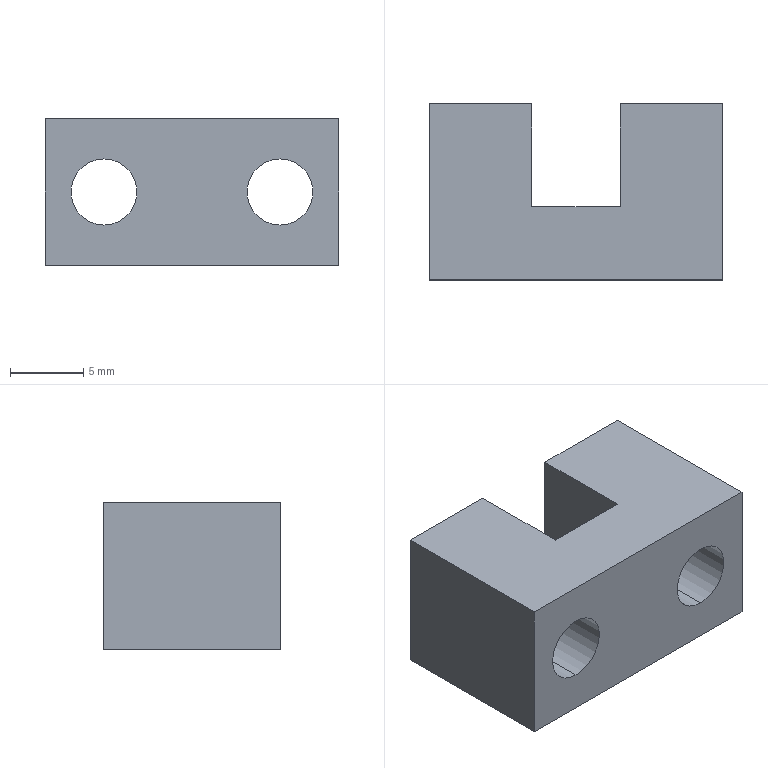Part | STEP file | insert limit | 1 solid | 17 faces | box 20 x 12 x 10 mm | volume 1551 mm3 | plane 11 | cylinder 6 | commonest cylinder face diameters 4.5 x6
STEP:
#1=CARTESIAN_POINT('',(0.,0.,0.));
#2=DIRECTION('',(0.,0.,1.));
#3=DIRECTION('',(1.,0.,0.));
#4=AXIS2_PLACEMENT_3D('',#1,#2,#3);
#5=CARTESIAN_POINT('',(0.,-4.,7.25));
#6=VERTEX_POINT('',#5);
#7=CARTESIAN_POINT('',(0.,-1.,7.25));
#8=VERTEX_POINT('',#7);
#9=CARTESIAN_POINT('',(0.,-12.364,7.25));
#10=DIRECTION('',(0.,1.,0.));
#11=VECTOR('',#10,1.);
#12=LINE('',#9,#11);
#13=CARTESIAN_POINT('',(0.,-12.364,5.));
#14=DIRECTION('',(0.,1.,0.));
#15=DIRECTION('',(0.,0.,1.));
#16=AXIS2_PLACEMENT_3D('',#13,#14,#15);
#17=CYLINDRICAL_SURFACE('',#16,2.25);
#18=CARTESIAN_POINT('',(6.283,0.));
#19=DIRECTION('',(0.,1.));
#20=VECTOR('',#19,1.);
#21=LINE('',#18,#20);
#22=(GEOMETRIC_REPRESENTATION_CONTEXT(2)PARAMETRIC_REPRESENTATION_CONTEXT()REPRESENTATION_CONTEXT('',''));
#23=DEFINITIONAL_REPRESENTATION('',(#21),#22);
#24=PCURVE('',#17,#23);
#25=CARTESIAN_POINT('',(0.,-12.364,5.));
#26=DIRECTION('',(0.,1.,0.));
#27=DIRECTION('',(0.,0.,1.));
#28=AXIS2_PLACEMENT_3D('',#25,#26,#27);
#29=CYLINDRICAL_SURFACE('',#28,2.25);
#30=CARTESIAN_POINT('',(0.,0.));
#31=DIRECTION('',(0.,1.));
#32=VECTOR('',#31,1.);
#33=LINE('',#30,#32);
#34=(GEOMETRIC_REPRESENTATION_CONTEXT(2)PARAMETRIC_REPRESENTATION_CONTEXT()REPRESENTATION_CONTEXT('',''));
#35=DEFINITIONAL_REPRESENTATION('',(#33),#34);
#36=PCURVE('',#29,#35);
#37=SURFACE_CURVE('',#12,(#24,#36),.PCURVE_S1.);
#38=EDGE_CURVE('',#6,#8,#37,.T.);
#39=ORIENTED_EDGE('',*,*,#38,.T.);
#40=CARTESIAN_POINT('',(0.,-1.,2.75));
#41=VERTEX_POINT('',#40);
#42=CARTESIAN_POINT('',(0.,-1.,5.));
#43=DIRECTION('',(0.,1.,0.));
#44=DIRECTION('',(0.,0.,1.));
#45=AXIS2_PLACEMENT_3D('',#42,#43,#44);
#46=CIRCLE('',#45,2.25);
#47=CARTESIAN_POINT('',(0.,11.364));
#48=DIRECTION('',(1.,0.));
#49=VECTOR('',#48,1.);
#50=LINE('',#47,#49);
#51=(GEOMETRIC_REPRESENTATION_CONTEXT(2)PARAMETRIC_REPRESENTATION_CONTEXT()REPRESENTATION_CONTEXT('',''));
#52=DEFINITIONAL_REPRESENTATION('',(#50),#51);
#53=PCURVE('',#17,#52);
#54=CARTESIAN_POINT('',(-3.,-1.,10.));
#55=DIRECTION('',(0.,-1.,0.));
#56=DIRECTION('',(0.,0.,-1.));
#57=AXIS2_PLACEMENT_3D('',#54,#55,#56);
#58=PLANE('',#57);
#59=CARTESIAN_POINT('',(2.75,3.));
#60=CARTESIAN_POINT('',(2.75,6.897));
#61=CARTESIAN_POINT('',(6.125,4.949));
#62=CARTESIAN_POINT('',(9.5,3.));
#63=CARTESIAN_POINT('',(6.125,1.051));
#64=CARTESIAN_POINT('',(2.75,-0.8971));
#65=CARTESIAN_POINT('',(2.75,3.));
#66=(BOUNDED_CURVE()B_SPLINE_CURVE(2,(#59,#60,#61,#62,#63,#64,#65),.UNSPECIFIED.,.T.,.F.)B_SPLINE_CURVE_WITH_KNOTS((1,2,2,2,2,1),(-2.094,0.,2.094,4.189,6.283,8.378),.UNSPECIFIED.)CURVE()GEOMETRIC_REPRESENTATION_ITEM()RATIONAL_B_SPLINE_CURVE((1.,0.5,1.,0.5,1.,0.5,1.))REPRESENTATION_ITEM(''));
#67=(GEOMETRIC_REPRESENTATION_CONTEXT(2)PARAMETRIC_REPRESENTATION_CONTEXT()REPRESENTATION_CONTEXT('',''));
#68=DEFINITIONAL_REPRESENTATION('',(#66),#67);
#69=PCURVE('',#58,#68);
#70=SURFACE_CURVE('',#46,(#53,#69),.PCURVE_S1.);
#71=EDGE_CURVE('',#41,#8,#70,.T.);
#72=ORIENTED_EDGE('',*,*,#71,.F.);
#73=CARTESIAN_POINT('',(0.,-4.,2.75));
#74=VERTEX_POINT('',#73);
#75=CARTESIAN_POINT('',(0.,-12.364,2.75));
#76=DIRECTION('',(0.,1.,0.));
#77=VECTOR('',#76,1.);
#78=LINE('',#75,#77);
#79=CARTESIAN_POINT('',(3.142,0.));
#80=DIRECTION('',(0.,1.));
#81=VECTOR('',#80,1.);
#82=LINE('',#79,#81);
#83=(GEOMETRIC_REPRESENTATION_CONTEXT(2)PARAMETRIC_REPRESENTATION_CONTEXT()REPRESENTATION_CONTEXT('',''));
#84=DEFINITIONAL_REPRESENTATION('',(#82),#83);
#85=PCURVE('',#17,#84);
#86=CARTESIAN_POINT('',(3.142,0.));
#87=DIRECTION('',(0.,1.));
#88=VECTOR('',#87,1.);
#89=LINE('',#86,#88);
#90=(GEOMETRIC_REPRESENTATION_CONTEXT(2)PARAMETRIC_REPRESENTATION_CONTEXT()REPRESENTATION_CONTEXT('',''));
#91=DEFINITIONAL_REPRESENTATION('',(#89),#90);
#92=PCURVE('',#29,#91);
#93=SURFACE_CURVE('',#78,(#85,#92),.PCURVE_S1.);
#94=EDGE_CURVE('',#74,#41,#93,.T.);
#95=ORIENTED_EDGE('',*,*,#94,.F.);
#96=CARTESIAN_POINT('',(0.,-4.,5.));
#97=DIRECTION('',(0.,-1.,0.));
#98=DIRECTION('',(0.,0.,1.));
#99=AXIS2_PLACEMENT_3D('',#96,#97,#98);
#100=CIRCLE('',#99,2.25);
#101=CARTESIAN_POINT('',(6.283,8.364));
#102=DIRECTION('',(-1.,0.));
#103=VECTOR('',#102,1.);
#104=LINE('',#101,#103);
#105=(GEOMETRIC_REPRESENTATION_CONTEXT(2)PARAMETRIC_REPRESENTATION_CONTEXT()REPRESENTATION_CONTEXT('',''));
#106=DEFINITIONAL_REPRESENTATION('',(#104),#105);
#107=PCURVE('',#17,#106);
#108=CARTESIAN_POINT('',(-10.,-4.,10.));
#109=DIRECTION('',(0.,1.,0.));
#110=DIRECTION('',(0.,0.,1.));
#111=AXIS2_PLACEMENT_3D('',#108,#109,#110);
#112=PLANE('',#111);
#113=CARTESIAN_POINT('',(-2.75,10.));
#114=CARTESIAN_POINT('',(-2.75,6.103));
#115=CARTESIAN_POINT('',(-6.125,8.051));
#116=CARTESIAN_POINT('',(-9.5,10.));
#117=CARTESIAN_POINT('',(-6.125,11.949));
#118=CARTESIAN_POINT('',(-2.75,13.897));
#119=CARTESIAN_POINT('',(-2.75,10.));
#120=(BOUNDED_CURVE()B_SPLINE_CURVE(2,(#113,#114,#115,#116,#117,#118,#119),.UNSPECIFIED.,.T.,.F.)B_SPLINE_CURVE_WITH_KNOTS((1,2,2,2,2,1),(-2.094,0.,2.094,4.189,6.283,8.378),.UNSPECIFIED.)CURVE()GEOMETRIC_REPRESENTATION_ITEM()RATIONAL_B_SPLINE_CURVE((1.,0.5,1.,0.5,1.,0.5,1.))REPRESENTATION_ITEM(''));
#121=(GEOMETRIC_REPRESENTATION_CONTEXT(2)PARAMETRIC_REPRESENTATION_CONTEXT()REPRESENTATION_CONTEXT('',''));
#122=DEFINITIONAL_REPRESENTATION('',(#120),#121);
#123=PCURVE('',#112,#122);
#124=SURFACE_CURVE('',#100,(#107,#123),.PCURVE_S1.);
#125=EDGE_CURVE('',#6,#74,#124,.T.);
#126=ORIENTED_EDGE('',*,*,#125,.F.);
#127=EDGE_LOOP('',(#39,#72,#95,#126));
#128=FACE_BOUND('',#127,.F.);
#129=ADVANCED_FACE('',(#128),#17,.F.);
#130=CARTESIAN_POINT('',(6.,6.,2.75));
#131=VERTEX_POINT('',#130);
#132=CARTESIAN_POINT('',(6.,-6.,2.75));
#133=VERTEX_POINT('',#132);
#134=CARTESIAN_POINT('',(6.,6.,2.75));
#135=DIRECTION('',(0.,-1.,0.));
#136=VECTOR('',#135,1.);
#137=LINE('',#134,#136);
#138=CARTESIAN_POINT('',(6.,6.,5.));
#139=DIRECTION('',(0.,-1.,0.));
#140=DIRECTION('',(0.,0.,-1.));
#141=AXIS2_PLACEMENT_3D('',#138,#139,#140);
#142=CYLINDRICAL_SURFACE('',#141,2.25);
#143=CARTESIAN_POINT('',(6.283,0.));
#144=DIRECTION('',(0.,1.));
#145=VECTOR('',#144,1.);
#146=LINE('',#143,#145);
#147=(GEOMETRIC_REPRESENTATION_CONTEXT(2)PARAMETRIC_REPRESENTATION_CONTEXT()REPRESENTATION_CONTEXT('',''));
#148=DEFINITIONAL_REPRESENTATION('',(#146),#147);
#149=PCURVE('',#142,#148);
#150=CARTESIAN_POINT('',(6.,6.,5.));
#151=DIRECTION('',(0.,-1.,0.));
#152=DIRECTION('',(0.,0.,-1.));
#153=AXIS2_PLACEMENT_3D('',#150,#151,#152);
#154=CYLINDRICAL_SURFACE('',#153,2.25);
#155=CARTESIAN_POINT('',(0.,0.));
#156=DIRECTION('',(0.,1.));
#157=VECTOR('',#156,1.);
#158=LINE('',#155,#157);
#159=(GEOMETRIC_REPRESENTATION_CONTEXT(2)PARAMETRIC_REPRESENTATION_CONTEXT()REPRESENTATION_CONTEXT('',''));
#160=DEFINITIONAL_REPRESENTATION('',(#158),#159);
#161=PCURVE('',#154,#160);
#162=SURFACE_CURVE('',#137,(#149,#161),.PCURVE_S1.);
#163=EDGE_CURVE('',#131,#133,#162,.T.);
#164=ORIENTED_EDGE('',*,*,#163,.T.);
#165=CARTESIAN_POINT('',(6.,-6.,7.25));
#166=VERTEX_POINT('',#165);
#167=CARTESIAN_POINT('',(6.,-6.,5.));
#168=DIRECTION('',(0.,-1.,0.));
#169=DIRECTION('',(0.,0.,-1.));
#170=AXIS2_PLACEMENT_3D('',#167,#168,#169);
#171=CIRCLE('',#170,2.25);
#172=CARTESIAN_POINT('',(0.,12.));
#173=DIRECTION('',(1.,0.));
#174=VECTOR('',#173,1.);
#175=LINE('',#172,#174);
#176=(GEOMETRIC_REPRESENTATION_CONTEXT(2)PARAMETRIC_REPRESENTATION_CONTEXT()REPRESENTATION_CONTEXT('',''));
#177=DEFINITIONAL_REPRESENTATION('',(#175),#176);
#178=PCURVE('',#142,#177);
#179=CARTESIAN_POINT('',(-10.,-6.,10.));
#180=DIRECTION('',(0.,1.,0.));
#181=DIRECTION('',(0.,0.,1.));
#182=AXIS2_PLACEMENT_3D('',#179,#180,#181);
#183=PLANE('',#182);
#184=CARTESIAN_POINT('',(-7.25,16.));
#185=CARTESIAN_POINT('',(-7.25,19.897));
#186=CARTESIAN_POINT('',(-3.875,17.949));
#187=CARTESIAN_POINT('',(-0.5,16.));
#188=CARTESIAN_POINT('',(-3.875,14.051));
#189=CARTESIAN_POINT('',(-7.25,12.103));
#190=CARTESIAN_POINT('',(-7.25,16.));
#191=(BOUNDED_CURVE()B_SPLINE_CURVE(2,(#184,#185,#186,#187,#188,#189,#190),.UNSPECIFIED.,.T.,.F.)B_SPLINE_CURVE_WITH_KNOTS((1,2,2,2,2,1),(-2.094,0.,2.094,4.189,6.283,8.378),.UNSPECIFIED.)CURVE()GEOMETRIC_REPRESENTATION_ITEM()RATIONAL_B_SPLINE_CURVE((1.,0.5,1.,0.5,1.,0.5,1.))REPRESENTATION_ITEM(''));
#192=(GEOMETRIC_REPRESENTATION_CONTEXT(2)PARAMETRIC_REPRESENTATION_CONTEXT()REPRESENTATION_CONTEXT('',''));
#193=DEFINITIONAL_REPRESENTATION('',(#191),#192);
#194=PCURVE('',#183,#193);
#195=SURFACE_CURVE('',#171,(#178,#194),.PCURVE_S1.);
#196=EDGE_CURVE('',#166,#133,#195,.T.);
#197=ORIENTED_EDGE('',*,*,#196,.F.);
#198=CARTESIAN_POINT('',(6.,6.,7.25));
#199=VERTEX_POINT('',#198);
#200=CARTESIAN_POINT('',(6.,6.,7.25));
#201=DIRECTION('',(0.,-1.,0.));
#202=VECTOR('',#201,1.);
#203=LINE('',#200,#202);
#204=CARTESIAN_POINT('',(3.142,0.));
#205=DIRECTION('',(0.,1.));
#206=VECTOR('',#205,1.);
#207=LINE('',#204,#206);
#208=(GEOMETRIC_REPRESENTATION_CONTEXT(2)PARAMETRIC_REPRESENTATION_CONTEXT()REPRESENTATION_CONTEXT('',''));
#209=DEFINITIONAL_REPRESENTATION('',(#207),#208);
#210=PCURVE('',#142,#209);
#211=CARTESIAN_POINT('',(3.142,0.));
#212=DIRECTION('',(0.,1.));
#213=VECTOR('',#212,1.);
#214=LINE('',#211,#213);
#215=(GEOMETRIC_REPRESENTATION_CONTEXT(2)PARAMETRIC_REPRESENTATION_CONTEXT()REPRESENTATION_CONTEXT('',''));
#216=DEFINITIONAL_REPRESENTATION('',(#214),#215);
#217=PCURVE('',#154,#216);
#218=SURFACE_CURVE('',#203,(#210,#217),.PCURVE_S1.);
#219=EDGE_CURVE('',#199,#166,#218,.T.);
#220=ORIENTED_EDGE('',*,*,#219,.F.);
#221=CARTESIAN_POINT('',(6.,6.,5.));
#222=DIRECTION('',(0.,-1.,0.));
#223=DIRECTION('',(0.,0.,-1.));
#224=AXIS2_PLACEMENT_3D('',#221,#222,#223);
#225=CIRCLE('',#224,2.25);
#226=CARTESIAN_POINT('',(0.,0.));
#227=DIRECTION('',(1.,0.));
#228=VECTOR('',#227,1.);
#229=LINE('',#226,#228);
#230=(GEOMETRIC_REPRESENTATION_CONTEXT(2)PARAMETRIC_REPRESENTATION_CONTEXT()REPRESENTATION_CONTEXT('',''));
#231=DEFINITIONAL_REPRESENTATION('',(#229),#230);
#232=PCURVE('',#142,#231);
#233=CARTESIAN_POINT('',(3.,6.,10.));
#234=DIRECTION('',(0.,-1.,0.));
#235=DIRECTION('',(0.,0.,-1.));
#236=AXIS2_PLACEMENT_3D('',#233,#234,#235);
#237=PLANE('',#236);
#238=CARTESIAN_POINT('',(5.,3.));
#239=DIRECTION('',(1.,0.));
#240=AXIS2_PLACEMENT_2D('',#238,#239);
#241=CIRCLE('',#240,2.25);
#242=(GEOMETRIC_REPRESENTATION_CONTEXT(2)PARAMETRIC_REPRESENTATION_CONTEXT()REPRESENTATION_CONTEXT('',''));
#243=DEFINITIONAL_REPRESENTATION('',(#241),#242);
#244=PCURVE('',#237,#243);
#245=SURFACE_CURVE('',#225,(#232,#244),.PCURVE_S1.);
#246=EDGE_CURVE('',#199,#131,#245,.T.);
#247=ORIENTED_EDGE('',*,*,#246,.T.);
#248=EDGE_LOOP('',(#164,#197,#220,#247));
#249=FACE_BOUND('',#248,.F.);
#250=ADVANCED_FACE('',(#249),#142,.F.);
#251=CARTESIAN_POINT('',(-6.,6.,2.75));
#252=VERTEX_POINT('',#251);
#253=CARTESIAN_POINT('',(-6.,-6.,2.75));
#254=VERTEX_POINT('',#253);
#255=CARTESIAN_POINT('',(-6.,6.,2.75));
#256=DIRECTION('',(0.,-1.,0.));
#257=VECTOR('',#256,1.);
#258=LINE('',#255,#257);
#259=CARTESIAN_POINT('',(-6.,6.,5.));
#260=DIRECTION('',(0.,-1.,0.));
#261=DIRECTION('',(0.,0.,-1.));
#262=AXIS2_PLACEMENT_3D('',#259,#260,#261);
#263=CYLINDRICAL_SURFACE('',#262,2.25);
#264=CARTESIAN_POINT('',(6.283,0.));
#265=DIRECTION('',(0.,1.));
#266=VECTOR('',#265,1.);
#267=LINE('',#264,#266);
#268=(GEOMETRIC_REPRESENTATION_CONTEXT(2)PARAMETRIC_REPRESENTATION_CONTEXT()REPRESENTATION_CONTEXT('',''));
#269=DEFINITIONAL_REPRESENTATION('',(#267),#268);
#270=PCURVE('',#263,#269);
#271=CARTESIAN_POINT('',(-6.,6.,5.));
#272=DIRECTION('',(0.,-1.,0.));
#273=DIRECTION('',(0.,0.,-1.));
#274=AXIS2_PLACEMENT_3D('',#271,#272,#273);
#275=CYLINDRICAL_SURFACE('',#274,2.25);
#276=CARTESIAN_POINT('',(0.,0.));
#277=DIRECTION('',(0.,1.));
#278=VECTOR('',#277,1.);
#279=LINE('',#276,#278);
#280=(GEOMETRIC_REPRESENTATION_CONTEXT(2)PARAMETRIC_REPRESENTATION_CONTEXT()REPRESENTATION_CONTEXT('',''));
#281=DEFINITIONAL_REPRESENTATION('',(#279),#280);
#282=PCURVE('',#275,#281);
#283=SURFACE_CURVE('',#258,(#270,#282),.PCURVE_S1.);
#284=EDGE_CURVE('',#252,#254,#283,.T.);
#285=ORIENTED_EDGE('',*,*,#284,.T.);
#286=CARTESIAN_POINT('',(-6.,-6.,7.25));
#287=VERTEX_POINT('',#286);
#288=CARTESIAN_POINT('',(-6.,-6.,5.));
#289=DIRECTION('',(0.,-1.,0.));
#290=DIRECTION('',(0.,0.,-1.));
#291=AXIS2_PLACEMENT_3D('',#288,#289,#290);
#292=CIRCLE('',#291,2.25);
#293=CARTESIAN_POINT('',(0.,12.));
#294=DIRECTION('',(1.,0.));
#295=VECTOR('',#294,1.);
#296=LINE('',#293,#295);
#297=(GEOMETRIC_REPRESENTATION_CONTEXT(2)PARAMETRIC_REPRESENTATION_CONTEXT()REPRESENTATION_CONTEXT('',''));
#298=DEFINITIONAL_REPRESENTATION('',(#296),#297);
#299=PCURVE('',#263,#298);
#300=CARTESIAN_POINT('',(-7.25,4.));
#301=CARTESIAN_POINT('',(-7.25,7.897));
#302=CARTESIAN_POINT('',(-3.875,5.949));
#303=CARTESIAN_POINT('',(-0.5,4.));
#304=CARTESIAN_POINT('',(-3.875,2.051));
#305=CARTESIAN_POINT('',(-7.25,0.1029));
#306=CARTESIAN_POINT('',(-7.25,4.));
#307=(BOUNDED_CURVE()B_SPLINE_CURVE(2,(#300,#301,#302,#303,#304,#305,#306),.UNSPECIFIED.,.T.,.F.)B_SPLINE_CURVE_WITH_KNOTS((1,2,2,2,2,1),(-2.094,0.,2.094,4.189,6.283,8.378),.UNSPECIFIED.)CURVE()GEOMETRIC_REPRESENTATION_ITEM()RATIONAL_B_SPLINE_CURVE((1.,0.5,1.,0.5,1.,0.5,1.))REPRESENTATION_ITEM(''));
#308=(GEOMETRIC_REPRESENTATION_CONTEXT(2)PARAMETRIC_REPRESENTATION_CONTEXT()REPRESENTATION_CONTEXT('',''));
#309=DEFINITIONAL_REPRESENTATION('',(#307),#308);
#310=PCURVE('',#183,#309);
#311=SURFACE_CURVE('',#292,(#299,#310),.PCURVE_S1.);
#312=EDGE_CURVE('',#287,#254,#311,.T.);
#313=ORIENTED_EDGE('',*,*,#312,.F.);
#314=CARTESIAN_POINT('',(-6.,6.,7.25));
#315=VERTEX_POINT('',#314);
#316=CARTESIAN_POINT('',(-6.,6.,7.25));
#317=DIRECTION('',(0.,-1.,0.));
#318=VECTOR('',#317,1.);
#319=LINE('',#316,#318);
#320=CARTESIAN_POINT('',(3.142,0.));
#321=DIRECTION('',(0.,1.));
#322=VECTOR('',#321,1.);
#323=LINE('',#320,#322);
#324=(GEOMETRIC_REPRESENTATION_CONTEXT(2)PARAMETRIC_REPRESENTATION_CONTEXT()REPRESENTATION_CONTEXT('',''));
#325=DEFINITIONAL_REPRESENTATION('',(#323),#324);
#326=PCURVE('',#263,#325);
#327=CARTESIAN_POINT('',(3.142,0.));
#328=DIRECTION('',(0.,1.));
#329=VECTOR('',#328,1.);
#330=LINE('',#327,#329);
#331=(GEOMETRIC_REPRESENTATION_CONTEXT(2)PARAMETRIC_REPRESENTATION_CONTEXT()REPRESENTATION_CONTEXT('',''));
#332=DEFINITIONAL_REPRESENTATION('',(#330),#331);
#333=PCURVE('',#275,#332);
#334=SURFACE_CURVE('',#319,(#326,#333),.PCURVE_S1.);
#335=EDGE_CURVE('',#315,#287,#334,.T.);
#336=ORIENTED_EDGE('',*,*,#335,.F.);
#337=CARTESIAN_POINT('',(-6.,6.,5.));
#338=DIRECTION('',(0.,-1.,0.));
#339=DIRECTION('',(0.,0.,-1.));
#340=AXIS2_PLACEMENT_3D('',#337,#338,#339);
#341=CIRCLE('',#340,2.25);
#342=CARTESIAN_POINT('',(0.,0.));
#343=DIRECTION('',(1.,0.));
#344=VECTOR('',#343,1.);
#345=LINE('',#342,#344);
#346=(GEOMETRIC_REPRESENTATION_CONTEXT(2)PARAMETRIC_REPRESENTATION_CONTEXT()REPRESENTATION_CONTEXT('',''));
#347=DEFINITIONAL_REPRESENTATION('',(#345),#346);
#348=PCURVE('',#263,#347);
#349=CARTESIAN_POINT('',(-10.,6.,10.));
#350=DIRECTION('',(0.,-1.,0.));
#351=DIRECTION('',(0.,0.,-1.));
#352=AXIS2_PLACEMENT_3D('',#349,#350,#351);
#353=PLANE('',#352);
#354=CARTESIAN_POINT('',(5.,4.));
#355=DIRECTION('',(1.,0.));
#356=AXIS2_PLACEMENT_2D('',#354,#355);
#357=CIRCLE('',#356,2.25);
#358=(GEOMETRIC_REPRESENTATION_CONTEXT(2)PARAMETRIC_REPRESENTATION_CONTEXT()REPRESENTATION_CONTEXT('',''));
#359=DEFINITIONAL_REPRESENTATION('',(#357),#358);
#360=PCURVE('',#353,#359);
#361=SURFACE_CURVE('',#341,(#348,#360),.PCURVE_S1.);
#362=EDGE_CURVE('',#315,#252,#361,.T.);
#363=ORIENTED_EDGE('',*,*,#362,.T.);
#364=EDGE_LOOP('',(#285,#313,#336,#363));
#365=FACE_BOUND('',#364,.F.);
#366=ADVANCED_FACE('',(#365),#263,.F.);
#367=CARTESIAN_POINT('',(6.,6.,5.));
#368=DIRECTION('',(0.,-1.,0.));
#369=DIRECTION('',(0.,0.,-1.));
#370=AXIS2_PLACEMENT_3D('',#367,#368,#369);
#371=CIRCLE('',#370,2.25);
#372=CARTESIAN_POINT('',(5.,3.));
#373=DIRECTION('',(1.,0.));
#374=AXIS2_PLACEMENT_2D('',#372,#373);
#375=CIRCLE('',#374,2.25);
#376=(GEOMETRIC_REPRESENTATION_CONTEXT(2)PARAMETRIC_REPRESENTATION_CONTEXT()REPRESENTATION_CONTEXT('',''));
#377=DEFINITIONAL_REPRESENTATION('',(#375),#376);
#378=PCURVE('',#237,#377);
#379=CARTESIAN_POINT('',(0.,0.));
#380=DIRECTION('',(1.,0.));
#381=VECTOR('',#380,1.);
#382=LINE('',#379,#381);
#383=(GEOMETRIC_REPRESENTATION_CONTEXT(2)PARAMETRIC_REPRESENTATION_CONTEXT()REPRESENTATION_CONTEXT('',''));
#384=DEFINITIONAL_REPRESENTATION('',(#382),#383);
#385=PCURVE('',#154,#384);
#386=SURFACE_CURVE('',#371,(#378,#385),.PCURVE_S1.);
#387=EDGE_CURVE('',#131,#199,#386,.T.);
#388=ORIENTED_EDGE('',*,*,#387,.T.);
#389=ORIENTED_EDGE('',*,*,#246,.T.);
#390=EDGE_LOOP('',(#388,#389));
#391=FACE_BOUND('',#390,.T.);
#392=CARTESIAN_POINT('',(10.,6.,0.));
#393=VERTEX_POINT('',#392);
#394=CARTESIAN_POINT('',(3.,6.,0.));
#395=VERTEX_POINT('',#394);
#396=CARTESIAN_POINT('',(3.,6.,0.));
#397=DIRECTION('',(-1.,0.,0.));
#398=VECTOR('',#397,1.);
#399=LINE('',#396,#398);
#400=CARTESIAN_POINT('',(10.,0.));
#401=DIRECTION('',(0.,-1.));
#402=VECTOR('',#401,1.);
#403=LINE('',#400,#402);
#404=(GEOMETRIC_REPRESENTATION_CONTEXT(2)PARAMETRIC_REPRESENTATION_CONTEXT()REPRESENTATION_CONTEXT('',''));
#405=DEFINITIONAL_REPRESENTATION('',(#403),#404);
#406=PCURVE('',#237,#405);
#407=CARTESIAN_POINT('',(10.,6.,0.));
#408=DIRECTION('',(0.,0.,1.));
#409=DIRECTION('',(1.,0.,0.));
#410=AXIS2_PLACEMENT_3D('',#407,#408,#409);
#411=PLANE('',#410);
#412=CARTESIAN_POINT('',(-7.,0.));
#413=DIRECTION('',(-1.,0.));
#414=VECTOR('',#413,1.);
#415=LINE('',#412,#414);
#416=(GEOMETRIC_REPRESENTATION_CONTEXT(2)PARAMETRIC_REPRESENTATION_CONTEXT()REPRESENTATION_CONTEXT('',''));
#417=DEFINITIONAL_REPRESENTATION('',(#415),#416);
#418=PCURVE('',#411,#417);
#419=SURFACE_CURVE('',#399,(#406,#418),.PCURVE_S1.);
#420=EDGE_CURVE('',#393,#395,#419,.T.);
#421=ORIENTED_EDGE('',*,*,#420,.T.);
#422=CARTESIAN_POINT('',(3.,6.,10.));
#423=VERTEX_POINT('',#422);
#424=CARTESIAN_POINT('',(3.,6.,10.));
#425=DIRECTION('',(0.,0.,-1.));
#426=VECTOR('',#425,1.);
#427=LINE('',#424,#426);
#428=CARTESIAN_POINT('',(0.,0.));
#429=DIRECTION('',(1.,0.));
#430=VECTOR('',#429,1.);
#431=LINE('',#428,#430);
#432=(GEOMETRIC_REPRESENTATION_CONTEXT(2)PARAMETRIC_REPRESENTATION_CONTEXT()REPRESENTATION_CONTEXT('',''));
#433=DEFINITIONAL_REPRESENTATION('',(#431),#432);
#434=PCURVE('',#237,#433);
#435=CARTESIAN_POINT('',(3.,6.,10.));
#436=DIRECTION('',(1.,0.,0.));
#437=DIRECTION('',(0.,1.,0.));
#438=AXIS2_PLACEMENT_3D('',#435,#436,#437);
#439=PLANE('',#438);
#440=CARTESIAN_POINT('',(0.,0.));
#441=DIRECTION('',(0.,-1.));
#442=VECTOR('',#441,1.);
#443=LINE('',#440,#442);
#444=(GEOMETRIC_REPRESENTATION_CONTEXT(2)PARAMETRIC_REPRESENTATION_CONTEXT()REPRESENTATION_CONTEXT('',''));
#445=DEFINITIONAL_REPRESENTATION('',(#443),#444);
#446=PCURVE('',#439,#445);
#447=SURFACE_CURVE('',#427,(#434,#446),.PCURVE_S1.);
#448=EDGE_CURVE('',#423,#395,#447,.T.);
#449=ORIENTED_EDGE('',*,*,#448,.F.);
#450=CARTESIAN_POINT('',(10.,6.,10.));
#451=VERTEX_POINT('',#450);
#452=CARTESIAN_POINT('',(3.,6.,10.));
#453=DIRECTION('',(-1.,0.,0.));
#454=VECTOR('',#453,1.);
#455=LINE('',#452,#454);
#456=CARTESIAN_POINT('',(0.,0.));
#457=DIRECTION('',(0.,-1.));
#458=VECTOR('',#457,1.);
#459=LINE('',#456,#458);
#460=(GEOMETRIC_REPRESENTATION_CONTEXT(2)PARAMETRIC_REPRESENTATION_CONTEXT()REPRESENTATION_CONTEXT('',''));
#461=DEFINITIONAL_REPRESENTATION('',(#459),#460);
#462=PCURVE('',#237,#461);
#463=CARTESIAN_POINT('',(10.,6.,10.));
#464=DIRECTION('',(0.,0.,1.));
#465=DIRECTION('',(1.,0.,0.));
#466=AXIS2_PLACEMENT_3D('',#463,#464,#465);
#467=PLANE('',#466);
#468=CARTESIAN_POINT('',(-7.,0.));
#469=DIRECTION('',(-1.,0.));
#470=VECTOR('',#469,1.);
#471=LINE('',#468,#470);
#472=(GEOMETRIC_REPRESENTATION_CONTEXT(2)PARAMETRIC_REPRESENTATION_CONTEXT()REPRESENTATION_CONTEXT('',''));
#473=DEFINITIONAL_REPRESENTATION('',(#471),#472);
#474=PCURVE('',#467,#473);
#475=SURFACE_CURVE('',#455,(#462,#474),.PCURVE_S1.);
#476=EDGE_CURVE('',#451,#423,#475,.T.);
#477=ORIENTED_EDGE('',*,*,#476,.F.);
#478=CARTESIAN_POINT('',(10.,6.,10.));
#479=DIRECTION('',(0.,0.,-1.));
#480=VECTOR('',#479,1.);
#481=LINE('',#478,#480);
#482=CARTESIAN_POINT('',(0.,7.));
#483=DIRECTION('',(1.,0.));
#484=VECTOR('',#483,1.);
#485=LINE('',#482,#484);
#486=(GEOMETRIC_REPRESENTATION_CONTEXT(2)PARAMETRIC_REPRESENTATION_CONTEXT()REPRESENTATION_CONTEXT('',''));
#487=DEFINITIONAL_REPRESENTATION('',(#485),#486);
#488=PCURVE('',#237,#487);
#489=CARTESIAN_POINT('',(10.,-6.,10.));
#490=DIRECTION('',(-1.,0.,0.));
#491=DIRECTION('',(0.,0.,1.));
#492=AXIS2_PLACEMENT_3D('',#489,#490,#491);
#493=PLANE('',#492);
#494=CARTESIAN_POINT('',(0.,12.));
#495=DIRECTION('',(-1.,0.));
#496=VECTOR('',#495,1.);
#497=LINE('',#494,#496);
#498=(GEOMETRIC_REPRESENTATION_CONTEXT(2)PARAMETRIC_REPRESENTATION_CONTEXT()REPRESENTATION_CONTEXT('',''));
#499=DEFINITIONAL_REPRESENTATION('',(#497),#498);
#500=PCURVE('',#493,#499);
#501=SURFACE_CURVE('',#481,(#488,#500),.PCURVE_S1.);
#502=EDGE_CURVE('',#451,#393,#501,.T.);
#503=ORIENTED_EDGE('',*,*,#502,.T.);
#504=EDGE_LOOP('',(#421,#449,#477,#503));
#505=FACE_BOUND('',#504,.T.);
#506=ADVANCED_FACE('',(#391,#505),#237,.F.);
#507=CARTESIAN_POINT('',(3.,-1.,0.));
#508=VERTEX_POINT('',#507);
#509=CARTESIAN_POINT('',(3.,6.,0.));
#510=DIRECTION('',(0.,-1.,0.));
#511=VECTOR('',#510,1.);
#512=LINE('',#509,#511);
#513=CARTESIAN_POINT('',(0.,-10.));
#514=DIRECTION('',(-1.,0.));
#515=VECTOR('',#514,1.);
#516=LINE('',#513,#515);
#517=(GEOMETRIC_REPRESENTATION_CONTEXT(2)PARAMETRIC_REPRESENTATION_CONTEXT()REPRESENTATION_CONTEXT('',''));
#518=DEFINITIONAL_REPRESENTATION('',(#516),#517);
#519=PCURVE('',#439,#518);
#520=CARTESIAN_POINT('',(-7.,0.));
#521=DIRECTION('',(0.,-1.));
#522=VECTOR('',#521,1.);
#523=LINE('',#520,#522);
#524=(GEOMETRIC_REPRESENTATION_CONTEXT(2)PARAMETRIC_REPRESENTATION_CONTEXT()REPRESENTATION_CONTEXT('',''));
#525=DEFINITIONAL_REPRESENTATION('',(#523),#524);
#526=PCURVE('',#411,#525);
#527=SURFACE_CURVE('',#512,(#519,#526),.PCURVE_S1.);
#528=EDGE_CURVE('',#395,#508,#527,.T.);
#529=ORIENTED_EDGE('',*,*,#528,.T.);
#530=CARTESIAN_POINT('',(3.,-1.,10.));
#531=VERTEX_POINT('',#530);
#532=CARTESIAN_POINT('',(3.,-1.,10.));
#533=DIRECTION('',(0.,0.,-1.));
#534=VECTOR('',#533,1.);
#535=LINE('',#532,#534);
#536=CARTESIAN_POINT('',(-7.,0.));
#537=DIRECTION('',(0.,-1.));
#538=VECTOR('',#537,1.);
#539=LINE('',#536,#538);
#540=(GEOMETRIC_REPRESENTATION_CONTEXT(2)PARAMETRIC_REPRESENTATION_CONTEXT()REPRESENTATION_CONTEXT('',''));
#541=DEFINITIONAL_REPRESENTATION('',(#539),#540);
#542=PCURVE('',#439,#541);
#543=CARTESIAN_POINT('',(0.,6.));
#544=DIRECTION('',(1.,0.));
#545=VECTOR('',#544,1.);
#546=LINE('',#543,#545);
#547=(GEOMETRIC_REPRESENTATION_CONTEXT(2)PARAMETRIC_REPRESENTATION_CONTEXT()REPRESENTATION_CONTEXT('',''));
#548=DEFINITIONAL_REPRESENTATION('',(#546),#547);
#549=PCURVE('',#58,#548);
#550=SURFACE_CURVE('',#535,(#542,#549),.PCURVE_S1.);
#551=EDGE_CURVE('',#531,#508,#550,.T.);
#552=ORIENTED_EDGE('',*,*,#551,.F.);
#553=CARTESIAN_POINT('',(3.,6.,10.));
#554=DIRECTION('',(0.,-1.,0.));
#555=VECTOR('',#554,1.);
#556=LINE('',#553,#555);
#557=CARTESIAN_POINT('',(0.,0.));
#558=DIRECTION('',(-1.,0.));
#559=VECTOR('',#558,1.);
#560=LINE('',#557,#559);
#561=(GEOMETRIC_REPRESENTATION_CONTEXT(2)PARAMETRIC_REPRESENTATION_CONTEXT()REPRESENTATION_CONTEXT('',''));
#562=DEFINITIONAL_REPRESENTATION('',(#560),#561);
#563=PCURVE('',#439,#562);
#564=CARTESIAN_POINT('',(-7.,0.));
#565=DIRECTION('',(0.,-1.));
#566=VECTOR('',#565,1.);
#567=LINE('',#564,#566);
#568=(GEOMETRIC_REPRESENTATION_CONTEXT(2)PARAMETRIC_REPRESENTATION_CONTEXT()REPRESENTATION_CONTEXT('',''));
#569=DEFINITIONAL_REPRESENTATION('',(#567),#568);
#570=PCURVE('',#467,#569);
#571=SURFACE_CURVE('',#556,(#563,#570),.PCURVE_S1.);
#572=EDGE_CURVE('',#423,#531,#571,.T.);
#573=ORIENTED_EDGE('',*,*,#572,.F.);
#574=ORIENTED_EDGE('',*,*,#448,.T.);
#575=EDGE_LOOP('',(#529,#552,#573,#574));
#576=FACE_BOUND('',#575,.T.);
#577=ADVANCED_FACE('',(#576),#439,.F.);
#578=CARTESIAN_POINT('',(0.,-1.,5.));
#579=DIRECTION('',(0.,1.,0.));
#580=DIRECTION('',(0.,0.,1.));
#581=AXIS2_PLACEMENT_3D('',#578,#579,#580);
#582=CIRCLE('',#581,2.25);
#583=CARTESIAN_POINT('',(2.75,3.));
#584=CARTESIAN_POINT('',(2.75,6.897));
#585=CARTESIAN_POINT('',(6.125,4.949));
#586=CARTESIAN_POINT('',(9.5,3.));
#587=CARTESIAN_POINT('',(6.125,1.051));
#588=CARTESIAN_POINT('',(2.75,-0.8971));
#589=CARTESIAN_POINT('',(2.75,3.));
#590=(BOUNDED_CURVE()B_SPLINE_CURVE(2,(#583,#584,#585,#586,#587,#588,#589),.UNSPECIFIED.,.T.,.F.)B_SPLINE_CURVE_WITH_KNOTS((1,2,2,2,2,1),(-2.094,0.,2.094,4.189,6.283,8.378),.UNSPECIFIED.)CURVE()GEOMETRIC_REPRESENTATION_ITEM()RATIONAL_B_SPLINE_CURVE((1.,0.5,1.,0.5,1.,0.5,1.))REPRESENTATION_ITEM(''));
#591=(GEOMETRIC_REPRESENTATION_CONTEXT(2)PARAMETRIC_REPRESENTATION_CONTEXT()REPRESENTATION_CONTEXT('',''));
#592=DEFINITIONAL_REPRESENTATION('',(#590),#591);
#593=PCURVE('',#58,#592);
#594=CARTESIAN_POINT('',(0.,11.364));
#595=DIRECTION('',(1.,0.));
#596=VECTOR('',#595,1.);
#597=LINE('',#594,#596);
#598=(GEOMETRIC_REPRESENTATION_CONTEXT(2)PARAMETRIC_REPRESENTATION_CONTEXT()REPRESENTATION_CONTEXT('',''));
#599=DEFINITIONAL_REPRESENTATION('',(#597),#598);
#600=PCURVE('',#29,#599);
#601=SURFACE_CURVE('',#582,(#593,#600),.PCURVE_S1.);
#602=EDGE_CURVE('',#8,#41,#601,.T.);
#603=ORIENTED_EDGE('',*,*,#602,.F.);
#604=ORIENTED_EDGE('',*,*,#71,.F.);
#605=EDGE_LOOP('',(#603,#604));
#606=FACE_BOUND('',#605,.T.);
#607=CARTESIAN_POINT('',(-3.,-1.,0.));
#608=VERTEX_POINT('',#607);
#609=CARTESIAN_POINT('',(-3.,-1.,0.));
#610=DIRECTION('',(-1.,0.,0.));
#611=VECTOR('',#610,1.);
#612=LINE('',#609,#611);
#613=CARTESIAN_POINT('',(10.,0.));
#614=DIRECTION('',(0.,-1.));
#615=VECTOR('',#614,1.);
#616=LINE('',#613,#615);
#617=(GEOMETRIC_REPRESENTATION_CONTEXT(2)PARAMETRIC_REPRESENTATION_CONTEXT()REPRESENTATION_CONTEXT('',''));
#618=DEFINITIONAL_REPRESENTATION('',(#616),#617);
#619=PCURVE('',#58,#618);
#620=CARTESIAN_POINT('',(-13.,-7.));
#621=DIRECTION('',(-1.,0.));
#622=VECTOR('',#621,1.);
#623=LINE('',#620,#622);
#624=(GEOMETRIC_REPRESENTATION_CONTEXT(2)PARAMETRIC_REPRESENTATION_CONTEXT()REPRESENTATION_CONTEXT('',''));
#625=DEFINITIONAL_REPRESENTATION('',(#623),#624);
#626=PCURVE('',#411,#625);
#627=SURFACE_CURVE('',#612,(#619,#626),.PCURVE_S1.);
#628=EDGE_CURVE('',#508,#608,#627,.T.);
#629=ORIENTED_EDGE('',*,*,#628,.T.);
#630=CARTESIAN_POINT('',(-3.,-1.,10.));
#631=VERTEX_POINT('',#630);
#632=CARTESIAN_POINT('',(-3.,-1.,10.));
#633=DIRECTION('',(0.,0.,-1.));
#634=VECTOR('',#633,1.);
#635=LINE('',#632,#634);
#636=CARTESIAN_POINT('',(0.,0.));
#637=DIRECTION('',(1.,0.));
#638=VECTOR('',#637,1.);
#639=LINE('',#636,#638);
#640=(GEOMETRIC_REPRESENTATION_CONTEXT(2)PARAMETRIC_REPRESENTATION_CONTEXT()REPRESENTATION_CONTEXT('',''));
#641=DEFINITIONAL_REPRESENTATION('',(#639),#640);
#642=PCURVE('',#58,#641);
#643=CARTESIAN_POINT('',(-3.,6.,10.));
#644=DIRECTION('',(-1.,0.,0.));
#645=DIRECTION('',(0.,-1.,0.));
#646=AXIS2_PLACEMENT_3D('',#643,#644,#645);
#647=PLANE('',#646);
#648=CARTESIAN_POINT('',(7.,0.));
#649=DIRECTION('',(0.,-1.));
#650=VECTOR('',#649,1.);
#651=LINE('',#648,#650);
#652=(GEOMETRIC_REPRESENTATION_CONTEXT(2)PARAMETRIC_REPRESENTATION_CONTEXT()REPRESENTATION_CONTEXT('',''));
#653=DEFINITIONAL_REPRESENTATION('',(#651),#652);
#654=PCURVE('',#647,#653);
#655=SURFACE_CURVE('',#635,(#642,#654),.PCURVE_S1.);
#656=EDGE_CURVE('',#631,#608,#655,.T.);
#657=ORIENTED_EDGE('',*,*,#656,.F.);
#658=CARTESIAN_POINT('',(-3.,-1.,10.));
#659=DIRECTION('',(-1.,0.,0.));
#660=VECTOR('',#659,1.);
#661=LINE('',#658,#660);
#662=CARTESIAN_POINT('',(0.,0.));
#663=DIRECTION('',(0.,-1.));
#664=VECTOR('',#663,1.);
#665=LINE('',#662,#664);
#666=(GEOMETRIC_REPRESENTATION_CONTEXT(2)PARAMETRIC_REPRESENTATION_CONTEXT()REPRESENTATION_CONTEXT('',''));
#667=DEFINITIONAL_REPRESENTATION('',(#665),#666);
#668=PCURVE('',#58,#667);
#669=CARTESIAN_POINT('',(-13.,-7.));
#670=DIRECTION('',(-1.,0.));
#671=VECTOR('',#670,1.);
#672=LINE('',#669,#671);
#673=(GEOMETRIC_REPRESENTATION_CONTEXT(2)PARAMETRIC_REPRESENTATION_CONTEXT()REPRESENTATION_CONTEXT('',''));
#674=DEFINITIONAL_REPRESENTATION('',(#672),#673);
#675=PCURVE('',#467,#674);
#676=SURFACE_CURVE('',#661,(#668,#675),.PCURVE_S1.);
#677=EDGE_CURVE('',#531,#631,#676,.T.);
#678=ORIENTED_EDGE('',*,*,#677,.F.);
#679=ORIENTED_EDGE('',*,*,#551,.T.);
#680=EDGE_LOOP('',(#629,#657,#678,#679));
#681=FACE_BOUND('',#680,.T.);
#682=ADVANCED_FACE('',(#606,#681),#58,.F.);
#683=CARTESIAN_POINT('',(-3.,6.,0.));
#684=VERTEX_POINT('',#683);
#685=CARTESIAN_POINT('',(-3.,6.,0.));
#686=DIRECTION('',(0.,1.,0.));
#687=VECTOR('',#686,1.);
#688=LINE('',#685,#687);
#689=CARTESIAN_POINT('',(0.,-10.));
#690=DIRECTION('',(-1.,0.));
#691=VECTOR('',#690,1.);
#692=LINE('',#689,#691);
#693=(GEOMETRIC_REPRESENTATION_CONTEXT(2)PARAMETRIC_REPRESENTATION_CONTEXT()REPRESENTATION_CONTEXT('',''));
#694=DEFINITIONAL_REPRESENTATION('',(#692),#693);
#695=PCURVE('',#647,#694);
#696=CARTESIAN_POINT('',(-13.,0.));
#697=DIRECTION('',(0.,1.));
#698=VECTOR('',#697,1.);
#699=LINE('',#696,#698);
#700=(GEOMETRIC_REPRESENTATION_CONTEXT(2)PARAMETRIC_REPRESENTATION_CONTEXT()REPRESENTATION_CONTEXT('',''));
#701=DEFINITIONAL_REPRESENTATION('',(#699),#700);
#702=PCURVE('',#411,#701);
#703=SURFACE_CURVE('',#688,(#695,#702),.PCURVE_S1.);
#704=EDGE_CURVE('',#608,#684,#703,.T.);
#705=ORIENTED_EDGE('',*,*,#704,.T.);
#706=CARTESIAN_POINT('',(-3.,6.,10.));
#707=VERTEX_POINT('',#706);
#708=CARTESIAN_POINT('',(-3.,6.,10.));
#709=DIRECTION('',(0.,0.,-1.));
#710=VECTOR('',#709,1.);
#711=LINE('',#708,#710);
#712=CARTESIAN_POINT('',(0.,0.));
#713=DIRECTION('',(0.,-1.));
#714=VECTOR('',#713,1.);
#715=LINE('',#712,#714);
#716=(GEOMETRIC_REPRESENTATION_CONTEXT(2)PARAMETRIC_REPRESENTATION_CONTEXT()REPRESENTATION_CONTEXT('',''));
#717=DEFINITIONAL_REPRESENTATION('',(#715),#716);
#718=PCURVE('',#647,#717);
#719=CARTESIAN_POINT('',(0.,7.));
#720=DIRECTION('',(1.,0.));
#721=VECTOR('',#720,1.);
#722=LINE('',#719,#721);
#723=(GEOMETRIC_REPRESENTATION_CONTEXT(2)PARAMETRIC_REPRESENTATION_CONTEXT()REPRESENTATION_CONTEXT('',''));
#724=DEFINITIONAL_REPRESENTATION('',(#722),#723);
#725=PCURVE('',#353,#724);
#726=SURFACE_CURVE('',#711,(#718,#725),.PCURVE_S1.);
#727=EDGE_CURVE('',#707,#684,#726,.T.);
#728=ORIENTED_EDGE('',*,*,#727,.F.);
#729=CARTESIAN_POINT('',(-3.,6.,10.));
#730=DIRECTION('',(0.,1.,0.));
#731=VECTOR('',#730,1.);
#732=LINE('',#729,#731);
#733=CARTESIAN_POINT('',(0.,0.));
#734=DIRECTION('',(-1.,0.));
#735=VECTOR('',#734,1.);
#736=LINE('',#733,#735);
#737=(GEOMETRIC_REPRESENTATION_CONTEXT(2)PARAMETRIC_REPRESENTATION_CONTEXT()REPRESENTATION_CONTEXT('',''));
#738=DEFINITIONAL_REPRESENTATION('',(#736),#737);
#739=PCURVE('',#647,#738);
#740=CARTESIAN_POINT('',(-13.,0.));
#741=DIRECTION('',(0.,1.));
#742=VECTOR('',#741,1.);
#743=LINE('',#740,#742);
#744=(GEOMETRIC_REPRESENTATION_CONTEXT(2)PARAMETRIC_REPRESENTATION_CONTEXT()REPRESENTATION_CONTEXT('',''));
#745=DEFINITIONAL_REPRESENTATION('',(#743),#744);
#746=PCURVE('',#467,#745);
#747=SURFACE_CURVE('',#732,(#739,#746),.PCURVE_S1.);
#748=EDGE_CURVE('',#631,#707,#747,.T.);
#749=ORIENTED_EDGE('',*,*,#748,.F.);
#750=ORIENTED_EDGE('',*,*,#656,.T.);
#751=EDGE_LOOP('',(#705,#728,#749,#750));
#752=FACE_BOUND('',#751,.T.);
#753=ADVANCED_FACE('',(#752),#647,.F.);
#754=CARTESIAN_POINT('',(-6.,6.,5.));
#755=DIRECTION('',(0.,-1.,0.));
#756=DIRECTION('',(0.,0.,-1.));
#757=AXIS2_PLACEMENT_3D('',#754,#755,#756);
#758=CIRCLE('',#757,2.25);
#759=CARTESIAN_POINT('',(5.,4.));
#760=DIRECTION('',(1.,0.));
#761=AXIS2_PLACEMENT_2D('',#759,#760);
#762=CIRCLE('',#761,2.25);
#763=(GEOMETRIC_REPRESENTATION_CONTEXT(2)PARAMETRIC_REPRESENTATION_CONTEXT()REPRESENTATION_CONTEXT('',''));
#764=DEFINITIONAL_REPRESENTATION('',(#762),#763);
#765=PCURVE('',#353,#764);
#766=CARTESIAN_POINT('',(0.,0.));
#767=DIRECTION('',(1.,0.));
#768=VECTOR('',#767,1.);
#769=LINE('',#766,#768);
#770=(GEOMETRIC_REPRESENTATION_CONTEXT(2)PARAMETRIC_REPRESENTATION_CONTEXT()REPRESENTATION_CONTEXT('',''));
#771=DEFINITIONAL_REPRESENTATION('',(#769),#770);
#772=PCURVE('',#275,#771);
#773=SURFACE_CURVE('',#758,(#765,#772),.PCURVE_S1.);
#774=EDGE_CURVE('',#252,#315,#773,.T.);
#775=ORIENTED_EDGE('',*,*,#774,.T.);
#776=ORIENTED_EDGE('',*,*,#362,.T.);
#777=EDGE_LOOP('',(#775,#776));
#778=FACE_BOUND('',#777,.T.);
#779=CARTESIAN_POINT('',(-10.,6.,0.));
#780=VERTEX_POINT('',#779);
#781=CARTESIAN_POINT('',(-10.,6.,0.));
#782=DIRECTION('',(-1.,0.,0.));
#783=VECTOR('',#782,1.);
#784=LINE('',#781,#783);
#785=CARTESIAN_POINT('',(10.,0.));
#786=DIRECTION('',(0.,-1.));
#787=VECTOR('',#786,1.);
#788=LINE('',#785,#787);
#789=(GEOMETRIC_REPRESENTATION_CONTEXT(2)PARAMETRIC_REPRESENTATION_CONTEXT()REPRESENTATION_CONTEXT('',''));
#790=DEFINITIONAL_REPRESENTATION('',(#788),#789);
#791=PCURVE('',#353,#790);
#792=CARTESIAN_POINT('',(-20.,0.));
#793=DIRECTION('',(-1.,0.));
#794=VECTOR('',#793,1.);
#795=LINE('',#792,#794);
#796=(GEOMETRIC_REPRESENTATION_CONTEXT(2)PARAMETRIC_REPRESENTATION_CONTEXT()REPRESENTATION_CONTEXT('',''));
#797=DEFINITIONAL_REPRESENTATION('',(#795),#796);
#798=PCURVE('',#411,#797);
#799=SURFACE_CURVE('',#784,(#791,#798),.PCURVE_S1.);
#800=EDGE_CURVE('',#684,#780,#799,.T.);
#801=ORIENTED_EDGE('',*,*,#800,.T.);
#802=CARTESIAN_POINT('',(-10.,6.,10.));
#803=VERTEX_POINT('',#802);
#804=CARTESIAN_POINT('',(-10.,6.,10.));
#805=DIRECTION('',(0.,0.,-1.));
#806=VECTOR('',#805,1.);
#807=LINE('',#804,#806);
#808=CARTESIAN_POINT('',(0.,0.));
#809=DIRECTION('',(1.,0.));
#810=VECTOR('',#809,1.);
#811=LINE('',#808,#810);
#812=(GEOMETRIC_REPRESENTATION_CONTEXT(2)PARAMETRIC_REPRESENTATION_CONTEXT()REPRESENTATION_CONTEXT('',''));
#813=DEFINITIONAL_REPRESENTATION('',(#811),#812);
#814=PCURVE('',#353,#813);
#815=CARTESIAN_POINT('',(-10.,-6.,10.));
#816=DIRECTION('',(1.,0.,0.));
#817=DIRECTION('',(0.,0.,-1.));
#818=AXIS2_PLACEMENT_3D('',#815,#816,#817);
#819=PLANE('',#818);
#820=CARTESIAN_POINT('',(0.,12.));
#821=DIRECTION('',(1.,0.));
#822=VECTOR('',#821,1.);
#823=LINE('',#820,#822);
#824=(GEOMETRIC_REPRESENTATION_CONTEXT(2)PARAMETRIC_REPRESENTATION_CONTEXT()REPRESENTATION_CONTEXT('',''));
#825=DEFINITIONAL_REPRESENTATION('',(#823),#824);
#826=PCURVE('',#819,#825);
#827=SURFACE_CURVE('',#807,(#814,#826),.PCURVE_S1.);
#828=EDGE_CURVE('',#803,#780,#827,.T.);
#829=ORIENTED_EDGE('',*,*,#828,.F.);
#830=CARTESIAN_POINT('',(-10.,6.,10.));
#831=DIRECTION('',(-1.,0.,0.));
#832=VECTOR('',#831,1.);
#833=LINE('',#830,#832);
#834=CARTESIAN_POINT('',(0.,0.));
#835=DIRECTION('',(0.,-1.));
#836=VECTOR('',#835,1.);
#837=LINE('',#834,#836);
#838=(GEOMETRIC_REPRESENTATION_CONTEXT(2)PARAMETRIC_REPRESENTATION_CONTEXT()REPRESENTATION_CONTEXT('',''));
#839=DEFINITIONAL_REPRESENTATION('',(#837),#838);
#840=PCURVE('',#353,#839);
#841=CARTESIAN_POINT('',(-20.,0.));
#842=DIRECTION('',(-1.,0.));
#843=VECTOR('',#842,1.);
#844=LINE('',#841,#843);
#845=(GEOMETRIC_REPRESENTATION_CONTEXT(2)PARAMETRIC_REPRESENTATION_CONTEXT()REPRESENTATION_CONTEXT('',''));
#846=DEFINITIONAL_REPRESENTATION('',(#844),#845);
#847=PCURVE('',#467,#846);
#848=SURFACE_CURVE('',#833,(#840,#847),.PCURVE_S1.);
#849=EDGE_CURVE('',#707,#803,#848,.T.);
#850=ORIENTED_EDGE('',*,*,#849,.F.);
#851=ORIENTED_EDGE('',*,*,#727,.T.);
#852=EDGE_LOOP('',(#801,#829,#850,#851));
#853=FACE_BOUND('',#852,.T.);
#854=ADVANCED_FACE('',(#778,#853),#353,.F.);
#855=CARTESIAN_POINT('',(-10.,-6.,0.));
#856=VERTEX_POINT('',#855);
#857=CARTESIAN_POINT('',(-10.,-6.,0.));
#858=DIRECTION('',(0.,-1.,0.));
#859=VECTOR('',#858,1.);
#860=LINE('',#857,#859);
#861=CARTESIAN_POINT('',(10.,0.));
#862=DIRECTION('',(0.,-1.));
#863=VECTOR('',#862,1.);
#864=LINE('',#861,#863);
#865=(GEOMETRIC_REPRESENTATION_CONTEXT(2)PARAMETRIC_REPRESENTATION_CONTEXT()REPRESENTATION_CONTEXT('',''));
#866=DEFINITIONAL_REPRESENTATION('',(#864),#865);
#867=PCURVE('',#819,#866);
#868=CARTESIAN_POINT('',(-20.,-12.));
#869=DIRECTION('',(0.,-1.));
#870=VECTOR('',#869,1.);
#871=LINE('',#868,#870);
#872=(GEOMETRIC_REPRESENTATION_CONTEXT(2)PARAMETRIC_REPRESENTATION_CONTEXT()REPRESENTATION_CONTEXT('',''));
#873=DEFINITIONAL_REPRESENTATION('',(#871),#872);
#874=PCURVE('',#411,#873);
#875=SURFACE_CURVE('',#860,(#867,#874),.PCURVE_S1.);
#876=EDGE_CURVE('',#780,#856,#875,.T.);
#877=ORIENTED_EDGE('',*,*,#876,.T.);
#878=CARTESIAN_POINT('',(-10.,-6.,10.));
#879=VERTEX_POINT('',#878);
#880=CARTESIAN_POINT('',(-10.,-6.,10.));
#881=DIRECTION('',(0.,0.,-1.));
#882=VECTOR('',#881,1.);
#883=LINE('',#880,#882);
#884=CARTESIAN_POINT('',(0.,0.));
#885=DIRECTION('',(1.,0.));
#886=VECTOR('',#885,1.);
#887=LINE('',#884,#886);
#888=(GEOMETRIC_REPRESENTATION_CONTEXT(2)PARAMETRIC_REPRESENTATION_CONTEXT()REPRESENTATION_CONTEXT('',''));
#889=DEFINITIONAL_REPRESENTATION('',(#887),#888);
#890=PCURVE('',#819,#889);
#891=CARTESIAN_POINT('',(0.,0.));
#892=DIRECTION('',(-1.,0.));
#893=VECTOR('',#892,1.);
#894=LINE('',#891,#893);
#895=(GEOMETRIC_REPRESENTATION_CONTEXT(2)PARAMETRIC_REPRESENTATION_CONTEXT()REPRESENTATION_CONTEXT('',''));
#896=DEFINITIONAL_REPRESENTATION('',(#894),#895);
#897=PCURVE('',#183,#896);
#898=SURFACE_CURVE('',#883,(#890,#897),.PCURVE_S1.);
#899=EDGE_CURVE('',#879,#856,#898,.T.);
#900=ORIENTED_EDGE('',*,*,#899,.F.);
#901=CARTESIAN_POINT('',(-10.,-6.,10.));
#902=DIRECTION('',(0.,-1.,0.));
#903=VECTOR('',#902,1.);
#904=LINE('',#901,#903);
#905=CARTESIAN_POINT('',(0.,0.));
#906=DIRECTION('',(0.,-1.));
#907=VECTOR('',#906,1.);
#908=LINE('',#905,#907);
#909=(GEOMETRIC_REPRESENTATION_CONTEXT(2)PARAMETRIC_REPRESENTATION_CONTEXT()REPRESENTATION_CONTEXT('',''));
#910=DEFINITIONAL_REPRESENTATION('',(#908),#909);
#911=PCURVE('',#819,#910);
#912=CARTESIAN_POINT('',(-20.,-12.));
#913=DIRECTION('',(0.,-1.));
#914=VECTOR('',#913,1.);
#915=LINE('',#912,#914);
#916=(GEOMETRIC_REPRESENTATION_CONTEXT(2)PARAMETRIC_REPRESENTATION_CONTEXT()REPRESENTATION_CONTEXT('',''));
#917=DEFINITIONAL_REPRESENTATION('',(#915),#916);
#918=PCURVE('',#467,#917);
#919=SURFACE_CURVE('',#904,(#911,#918),.PCURVE_S1.);
#920=EDGE_CURVE('',#803,#879,#919,.T.);
#921=ORIENTED_EDGE('',*,*,#920,.F.);
#922=ORIENTED_EDGE('',*,*,#828,.T.);
#923=EDGE_LOOP('',(#877,#900,#921,#922));
#924=FACE_BOUND('',#923,.T.);
#925=ADVANCED_FACE('',(#924),#819,.F.);
#926=CARTESIAN_POINT('',(6.,-6.,5.));
#927=DIRECTION('',(0.,-1.,0.));
#928=DIRECTION('',(0.,0.,-1.));
#929=AXIS2_PLACEMENT_3D('',#926,#927,#928);
#930=CIRCLE('',#929,2.25);
#931=CARTESIAN_POINT('',(-7.25,16.));
#932=CARTESIAN_POINT('',(-7.25,19.897));
#933=CARTESIAN_POINT('',(-3.875,17.949));
#934=CARTESIAN_POINT('',(-0.5,16.));
#935=CARTESIAN_POINT('',(-3.875,14.051));
#936=CARTESIAN_POINT('',(-7.25,12.103));
#937=CARTESIAN_POINT('',(-7.25,16.));
#938=(BOUNDED_CURVE()B_SPLINE_CURVE(2,(#931,#932,#933,#934,#935,#936,#937),.UNSPECIFIED.,.T.,.F.)B_SPLINE_CURVE_WITH_KNOTS((1,2,2,2,2,1),(-2.094,0.,2.094,4.189,6.283,8.378),.UNSPECIFIED.)CURVE()GEOMETRIC_REPRESENTATION_ITEM()RATIONAL_B_SPLINE_CURVE((1.,0.5,1.,0.5,1.,0.5,1.))REPRESENTATION_ITEM(''));
#939=(GEOMETRIC_REPRESENTATION_CONTEXT(2)PARAMETRIC_REPRESENTATION_CONTEXT()REPRESENTATION_CONTEXT('',''));
#940=DEFINITIONAL_REPRESENTATION('',(#938),#939);
#941=PCURVE('',#183,#940);
#942=CARTESIAN_POINT('',(0.,12.));
#943=DIRECTION('',(1.,0.));
#944=VECTOR('',#943,1.);
#945=LINE('',#942,#944);
#946=(GEOMETRIC_REPRESENTATION_CONTEXT(2)PARAMETRIC_REPRESENTATION_CONTEXT()REPRESENTATION_CONTEXT('',''));
#947=DEFINITIONAL_REPRESENTATION('',(#945),#946);
#948=PCURVE('',#154,#947);
#949=SURFACE_CURVE('',#930,(#941,#948),.PCURVE_S1.);
#950=EDGE_CURVE('',#133,#166,#949,.T.);
#951=ORIENTED_EDGE('',*,*,#950,.F.);
#952=ORIENTED_EDGE('',*,*,#196,.F.);
#953=EDGE_LOOP('',(#951,#952));
#954=FACE_BOUND('',#953,.T.);
#955=CARTESIAN_POINT('',(-6.,-6.,5.));
#956=DIRECTION('',(0.,-1.,0.));
#957=DIRECTION('',(0.,0.,-1.));
#958=AXIS2_PLACEMENT_3D('',#955,#956,#957);
#959=CIRCLE('',#958,2.25);
#960=CARTESIAN_POINT('',(-7.25,4.));
#961=CARTESIAN_POINT('',(-7.25,7.897));
#962=CARTESIAN_POINT('',(-3.875,5.949));
#963=CARTESIAN_POINT('',(-0.5,4.));
#964=CARTESIAN_POINT('',(-3.875,2.051));
#965=CARTESIAN_POINT('',(-7.25,0.1029));
#966=CARTESIAN_POINT('',(-7.25,4.));
#967=(BOUNDED_CURVE()B_SPLINE_CURVE(2,(#960,#961,#962,#963,#964,#965,#966),.UNSPECIFIED.,.T.,.F.)B_SPLINE_CURVE_WITH_KNOTS((1,2,2,2,2,1),(-2.094,0.,2.094,4.189,6.283,8.378),.UNSPECIFIED.)CURVE()GEOMETRIC_REPRESENTATION_ITEM()RATIONAL_B_SPLINE_CURVE((1.,0.5,1.,0.5,1.,0.5,1.))REPRESENTATION_ITEM(''));
#968=(GEOMETRIC_REPRESENTATION_CONTEXT(2)PARAMETRIC_REPRESENTATION_CONTEXT()REPRESENTATION_CONTEXT('',''));
#969=DEFINITIONAL_REPRESENTATION('',(#967),#968);
#970=PCURVE('',#183,#969);
#971=CARTESIAN_POINT('',(0.,12.));
#972=DIRECTION('',(1.,0.));
#973=VECTOR('',#972,1.);
#974=LINE('',#971,#973);
#975=(GEOMETRIC_REPRESENTATION_CONTEXT(2)PARAMETRIC_REPRESENTATION_CONTEXT()REPRESENTATION_CONTEXT('',''));
#976=DEFINITIONAL_REPRESENTATION('',(#974),#975);
#977=PCURVE('',#275,#976);
#978=SURFACE_CURVE('',#959,(#970,#977),.PCURVE_S1.);
#979=EDGE_CURVE('',#254,#287,#978,.T.);
#980=ORIENTED_EDGE('',*,*,#979,.F.);
#981=ORIENTED_EDGE('',*,*,#312,.F.);
#982=EDGE_LOOP('',(#980,#981));
#983=FACE_BOUND('',#982,.T.);
#984=CARTESIAN_POINT('',(10.,-6.,0.));
#985=VERTEX_POINT('',#984);
#986=CARTESIAN_POINT('',(-10.,-6.,0.));
#987=DIRECTION('',(1.,0.,0.));
#988=VECTOR('',#987,1.);
#989=LINE('',#986,#988);
#990=CARTESIAN_POINT('',(-10.,0.));
#991=DIRECTION('',(0.,1.));
#992=VECTOR('',#991,1.);
#993=LINE('',#990,#992);
#994=(GEOMETRIC_REPRESENTATION_CONTEXT(2)PARAMETRIC_REPRESENTATION_CONTEXT()REPRESENTATION_CONTEXT('',''));
#995=DEFINITIONAL_REPRESENTATION('',(#993),#994);
#996=PCURVE('',#183,#995);
#997=CARTESIAN_POINT('',(-20.,-12.));
#998=DIRECTION('',(1.,0.));
#999=VECTOR('',#998,1.);
#1000=LINE('',#997,#999);
#1001=(GEOMETRIC_REPRESENTATION_CONTEXT(2)PARAMETRIC_REPRESENTATION_CONTEXT()REPRESENTATION_CONTEXT('',''));
#1002=DEFINITIONAL_REPRESENTATION('',(#1000),#1001);
#1003=PCURVE('',#411,#1002);
#1004=SURFACE_CURVE('',#989,(#996,#1003),.PCURVE_S1.);
#1005=EDGE_CURVE('',#856,#985,#1004,.T.);
#1006=ORIENTED_EDGE('',*,*,#1005,.T.);
#1007=CARTESIAN_POINT('',(10.,-6.,10.));
#1008=VERTEX_POINT('',#1007);
#1009=CARTESIAN_POINT('',(10.,-6.,10.));
#1010=DIRECTION('',(0.,0.,-1.));
#1011=VECTOR('',#1010,1.);
#1012=LINE('',#1009,#1011);
#1013=CARTESIAN_POINT('',(0.,20.));
#1014=DIRECTION('',(-1.,0.));
#1015=VECTOR('',#1014,1.);
#1016=LINE('',#1013,#1015);
#1017=(GEOMETRIC_REPRESENTATION_CONTEXT(2)PARAMETRIC_REPRESENTATION_CONTEXT()REPRESENTATION_CONTEXT('',''));
#1018=DEFINITIONAL_REPRESENTATION('',(#1016),#1017);
#1019=PCURVE('',#183,#1018);
#1020=CARTESIAN_POINT('',(0.,0.));
#1021=DIRECTION('',(-1.,0.));
#1022=VECTOR('',#1021,1.);
#1023=LINE('',#1020,#1022);
#1024=(GEOMETRIC_REPRESENTATION_CONTEXT(2)PARAMETRIC_REPRESENTATION_CONTEXT()REPRESENTATION_CONTEXT('',''));
#1025=DEFINITIONAL_REPRESENTATION('',(#1023),#1024);
#1026=PCURVE('',#493,#1025);
#1027=SURFACE_CURVE('',#1012,(#1019,#1026),.PCURVE_S1.);
#1028=EDGE_CURVE('',#1008,#985,#1027,.T.);
#1029=ORIENTED_EDGE('',*,*,#1028,.F.);
#1030=CARTESIAN_POINT('',(-10.,-6.,10.));
#1031=DIRECTION('',(1.,0.,0.));
#1032=VECTOR('',#1031,1.);
#1033=LINE('',#1030,#1032);
#1034=CARTESIAN_POINT('',(0.,0.));
#1035=DIRECTION('',(0.,1.));
#1036=VECTOR('',#1035,1.);
#1037=LINE('',#1034,#1036);
#1038=(GEOMETRIC_REPRESENTATION_CONTEXT(2)PARAMETRIC_REPRESENTATION_CONTEXT()REPRESENTATION_CONTEXT('',''));
#1039=DEFINITIONAL_REPRESENTATION('',(#1037),#1038);
#1040=PCURVE('',#183,#1039);
#1041=CARTESIAN_POINT('',(-20.,-12.));
#1042=DIRECTION('',(1.,0.));
#1043=VECTOR('',#1042,1.);
#1044=LINE('',#1041,#1043);
#1045=(GEOMETRIC_REPRESENTATION_CONTEXT(2)PARAMETRIC_REPRESENTATION_CONTEXT()REPRESENTATION_CONTEXT('',''));
#1046=DEFINITIONAL_REPRESENTATION('',(#1044),#1045);
#1047=PCURVE('',#467,#1046);
#1048=SURFACE_CURVE('',#1033,(#1040,#1047),.PCURVE_S1.);
#1049=EDGE_CURVE('',#879,#1008,#1048,.T.);
#1050=ORIENTED_EDGE('',*,*,#1049,.F.);
#1051=ORIENTED_EDGE('',*,*,#899,.T.);
#1052=EDGE_LOOP('',(#1006,#1029,#1050,#1051));
#1053=FACE_BOUND('',#1052,.T.);
#1054=ADVANCED_FACE('',(#954,#983,#1053),#183,.F.);
#1055=CARTESIAN_POINT('',(10.,-6.,0.));
#1056=DIRECTION('',(0.,1.,0.));
#1057=VECTOR('',#1056,1.);
#1058=LINE('',#1055,#1057);
#1059=CARTESIAN_POINT('',(-10.,0.));
#1060=DIRECTION('',(0.,1.));
#1061=VECTOR('',#1060,1.);
#1062=LINE('',#1059,#1061);
#1063=(GEOMETRIC_REPRESENTATION_CONTEXT(2)PARAMETRIC_REPRESENTATION_CONTEXT()REPRESENTATION_CONTEXT('',''));
#1064=DEFINITIONAL_REPRESENTATION('',(#1062),#1063);
#1065=PCURVE('',#493,#1064);
#1066=CARTESIAN_POINT('',(0.,-12.));
#1067=DIRECTION('',(0.,1.));
#1068=VECTOR('',#1067,1.);
#1069=LINE('',#1066,#1068);
#1070=(GEOMETRIC_REPRESENTATION_CONTEXT(2)PARAMETRIC_REPRESENTATION_CONTEXT()REPRESENTATION_CONTEXT('',''));
#1071=DEFINITIONAL_REPRESENTATION('',(#1069),#1070);
#1072=PCURVE('',#411,#1071);
#1073=SURFACE_CURVE('',#1058,(#1065,#1072),.PCURVE_S1.);
#1074=EDGE_CURVE('',#985,#393,#1073,.T.);
#1075=ORIENTED_EDGE('',*,*,#1074,.T.);
#1076=ORIENTED_EDGE('',*,*,#502,.F.);
#1077=CARTESIAN_POINT('',(10.,-6.,10.));
#1078=DIRECTION('',(0.,1.,0.));
#1079=VECTOR('',#1078,1.);
#1080=LINE('',#1077,#1079);
#1081=CARTESIAN_POINT('',(0.,0.));
#1082=DIRECTION('',(0.,1.));
#1083=VECTOR('',#1082,1.);
#1084=LINE('',#1081,#1083);
#1085=(GEOMETRIC_REPRESENTATION_CONTEXT(2)PARAMETRIC_REPRESENTATION_CONTEXT()REPRESENTATION_CONTEXT('',''));
#1086=DEFINITIONAL_REPRESENTATION('',(#1084),#1085);
#1087=PCURVE('',#493,#1086);
#1088=CARTESIAN_POINT('',(0.,-12.));
#1089=DIRECTION('',(0.,1.));
#1090=VECTOR('',#1089,1.);
#1091=LINE('',#1088,#1090);
#1092=(GEOMETRIC_REPRESENTATION_CONTEXT(2)PARAMETRIC_REPRESENTATION_CONTEXT()REPRESENTATION_CONTEXT('',''));
#1093=DEFINITIONAL_REPRESENTATION('',(#1091),#1092);
#1094=PCURVE('',#467,#1093);
#1095=SURFACE_CURVE('',#1080,(#1087,#1094),.PCURVE_S1.);
#1096=EDGE_CURVE('',#1008,#451,#1095,.T.);
#1097=ORIENTED_EDGE('',*,*,#1096,.F.);
#1098=ORIENTED_EDGE('',*,*,#1028,.T.);
#1099=EDGE_LOOP('',(#1075,#1076,#1097,#1098));
#1100=FACE_BOUND('',#1099,.T.);
#1101=ADVANCED_FACE('',(#1100),#493,.F.);
#1102=ORIENTED_EDGE('',*,*,#476,.T.);
#1103=ORIENTED_EDGE('',*,*,#572,.T.);
#1104=ORIENTED_EDGE('',*,*,#677,.T.);
#1105=ORIENTED_EDGE('',*,*,#748,.T.);
#1106=ORIENTED_EDGE('',*,*,#849,.T.);
#1107=ORIENTED_EDGE('',*,*,#920,.T.);
#1108=ORIENTED_EDGE('',*,*,#1049,.T.);
#1109=ORIENTED_EDGE('',*,*,#1096,.T.);
#1110=EDGE_LOOP('',(#1102,#1103,#1104,#1105,#1106,#1107,#1108,#1109));
#1111=FACE_BOUND('',#1110,.T.);
#1112=ADVANCED_FACE('',(#1111),#467,.T.);
#1113=ORIENTED_EDGE('',*,*,#420,.F.);
#1114=ORIENTED_EDGE('',*,*,#1074,.F.);
#1115=ORIENTED_EDGE('',*,*,#1005,.F.);
#1116=ORIENTED_EDGE('',*,*,#876,.F.);
#1117=ORIENTED_EDGE('',*,*,#800,.F.);
#1118=ORIENTED_EDGE('',*,*,#704,.F.);
#1119=ORIENTED_EDGE('',*,*,#628,.F.);
#1120=ORIENTED_EDGE('',*,*,#528,.F.);
#1121=EDGE_LOOP('',(#1113,#1114,#1115,#1116,#1117,#1118,#1119,#1120));
#1122=FACE_BOUND('',#1121,.T.);
#1123=ADVANCED_FACE('',(#1122),#411,.F.);
#1124=ORIENTED_EDGE('',*,*,#979,.F.);
#1125=ORIENTED_EDGE('',*,*,#284,.F.);
#1126=ORIENTED_EDGE('',*,*,#774,.T.);
#1127=ORIENTED_EDGE('',*,*,#335,.T.);
#1128=EDGE_LOOP('',(#1124,#1125,#1126,#1127));
#1129=FACE_BOUND('',#1128,.F.);
#1130=ADVANCED_FACE('',(#1129),#275,.F.);
#1131=ORIENTED_EDGE('',*,*,#950,.F.);
#1132=ORIENTED_EDGE('',*,*,#163,.F.);
#1133=ORIENTED_EDGE('',*,*,#387,.T.);
#1134=ORIENTED_EDGE('',*,*,#219,.T.);
#1135=EDGE_LOOP('',(#1131,#1132,#1133,#1134));
#1136=FACE_BOUND('',#1135,.F.);
#1137=ADVANCED_FACE('',(#1136),#154,.F.);
#1138=ORIENTED_EDGE('',*,*,#602,.F.);
#1139=ORIENTED_EDGE('',*,*,#38,.F.);
#1140=CARTESIAN_POINT('',(0.,-4.,5.));
#1141=DIRECTION('',(0.,-1.,0.));
#1142=DIRECTION('',(0.,0.,1.));
#1143=AXIS2_PLACEMENT_3D('',#1140,#1141,#1142);
#1144=CIRCLE('',#1143,2.25);
#1145=CARTESIAN_POINT('',(6.283,8.364));
#1146=DIRECTION('',(-1.,0.));
#1147=VECTOR('',#1146,1.);
#1148=LINE('',#1145,#1147);
#1149=(GEOMETRIC_REPRESENTATION_CONTEXT(2)PARAMETRIC_REPRESENTATION_CONTEXT()REPRESENTATION_CONTEXT('',''));
#1150=DEFINITIONAL_REPRESENTATION('',(#1148),#1149);
#1151=PCURVE('',#29,#1150);
#1152=CARTESIAN_POINT('',(-2.75,10.));
#1153=CARTESIAN_POINT('',(-2.75,6.103));
#1154=CARTESIAN_POINT('',(-6.125,8.051));
#1155=CARTESIAN_POINT('',(-9.5,10.));
#1156=CARTESIAN_POINT('',(-6.125,11.949));
#1157=CARTESIAN_POINT('',(-2.75,13.897));
#1158=CARTESIAN_POINT('',(-2.75,10.));
#1159=(BOUNDED_CURVE()B_SPLINE_CURVE(2,(#1152,#1153,#1154,#1155,#1156,#1157,#1158),.UNSPECIFIED.,.T.,.F.)B_SPLINE_CURVE_WITH_KNOTS((1,2,2,2,2,1),(-2.094,0.,2.094,4.189,6.283,8.378),.UNSPECIFIED.)CURVE()GEOMETRIC_REPRESENTATION_ITEM()RATIONAL_B_SPLINE_CURVE((1.,0.5,1.,0.5,1.,0.5,1.))REPRESENTATION_ITEM(''));
#1160=(GEOMETRIC_REPRESENTATION_CONTEXT(2)PARAMETRIC_REPRESENTATION_CONTEXT()REPRESENTATION_CONTEXT('',''));
#1161=DEFINITIONAL_REPRESENTATION('',(#1159),#1160);
#1162=PCURVE('',#112,#1161);
#1163=SURFACE_CURVE('',#1144,(#1151,#1162),.PCURVE_S1.);
#1164=EDGE_CURVE('',#74,#6,#1163,.T.);
#1165=ORIENTED_EDGE('',*,*,#1164,.F.);
#1166=ORIENTED_EDGE('',*,*,#94,.T.);
#1167=EDGE_LOOP('',(#1138,#1139,#1165,#1166));
#1168=FACE_BOUND('',#1167,.F.);
#1169=ADVANCED_FACE('',(#1168),#29,.F.);
#1170=ORIENTED_EDGE('',*,*,#125,.F.);
#1171=ORIENTED_EDGE('',*,*,#1164,.F.);
#1172=EDGE_LOOP('',(#1170,#1171));
#1173=FACE_BOUND('',#1172,.T.);
#1174=ADVANCED_FACE('',(#1173),#112,.T.);
#1175=CLOSED_SHELL('',(#129,#250,#366,#506,#577,#682,#753,#854,#925,#1054,#1101,#1112,#1123,#1130,#1137,#1169,#1174));
#1176=MANIFOLD_SOLID_BREP('',#1175);
#1177=(LENGTH_UNIT()NAMED_UNIT(*)SI_UNIT(.MILLI.,.METRE.));
#1178=UNCERTAINTY_MEASURE_WITH_UNIT(LENGTH_MEASURE(0.0000001),#1177,'','');
#1179=(NAMED_UNIT(*)PLANE_ANGLE_UNIT()SI_UNIT($,.RADIAN.));
#1180=(NAMED_UNIT(*)SI_UNIT($,.STERADIAN.)SOLID_ANGLE_UNIT());
#1181=(GEOMETRIC_REPRESENTATION_CONTEXT(3)GLOBAL_UNCERTAINTY_ASSIGNED_CONTEXT((#1178))GLOBAL_UNIT_ASSIGNED_CONTEXT((#1177,#1179,#1180))REPRESENTATION_CONTEXT('',''));
#1182=ADVANCED_BREP_SHAPE_REPRESENTATION('',(#4,#1176),#1181);